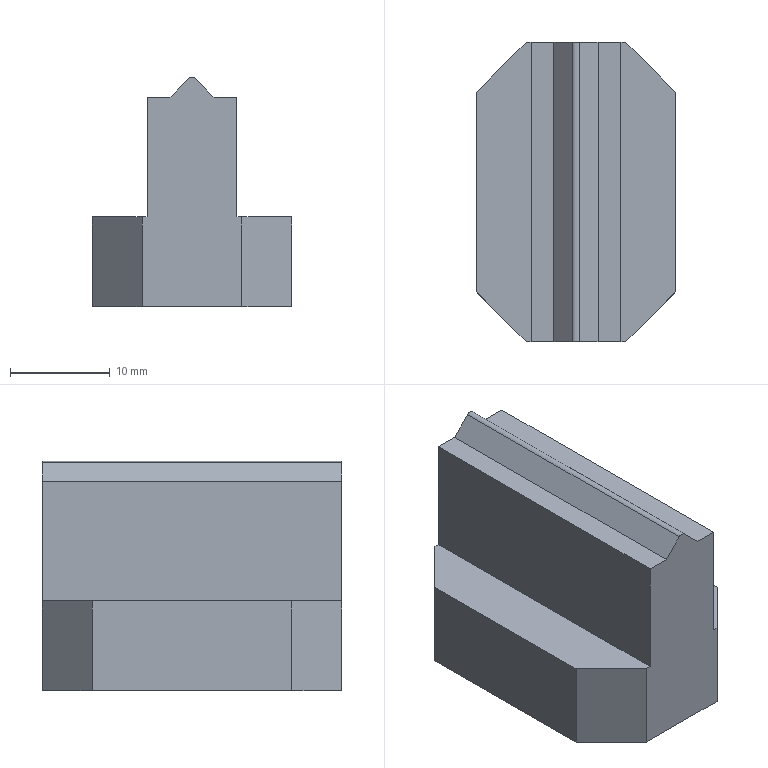Part | STEP file | lll_id382_x_t | 1 solid | 131 faces | box 20 x 30 x 23 mm | volume 8328 mm3 | plane 72 | other 58 | cylinder 1 | commonest cylinder face diameters 1 x1